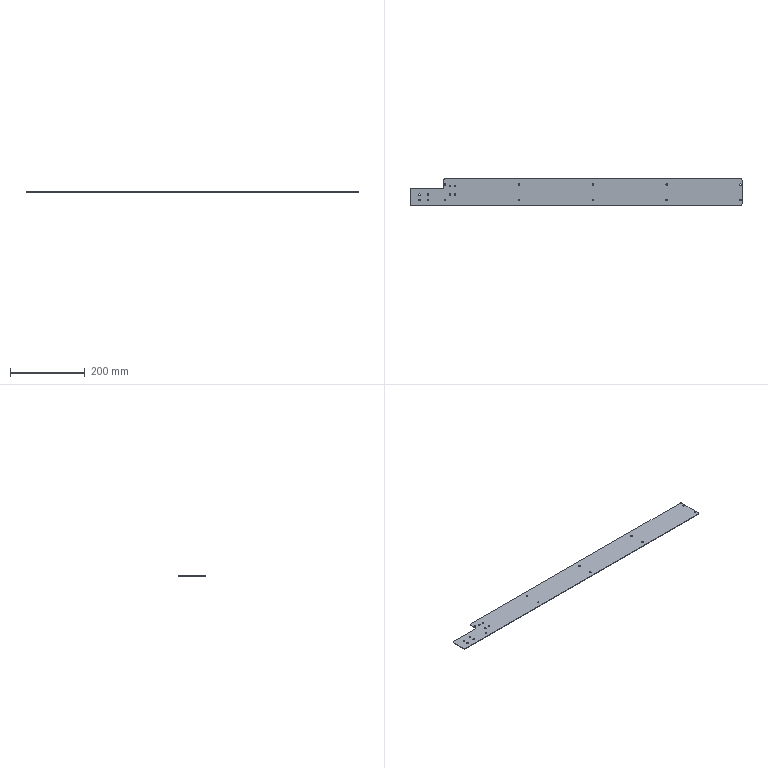Part | STEP file | SynoNew-0304-054 | 1 solid | 32 faces | box 890 x 70 x 1.5 mm | volume 89689 mm3 | cylinder 24 | plane 8 | commonest cylinder face diameters 4.2 x18 6 x6
STEP:
#1=CARTESIAN_POINT('',(-366.9,16.,1.5));
#2=VERTEX_POINT('',#1);
#3=CARTESIAN_POINT('',(-371.1,16.,1.5));
#4=VERTEX_POINT('',#3);
#5=CARTESIAN_POINT('',(-369.,16.,1.5));
#6=DIRECTION('',(0.,0.,-1.));
#7=DIRECTION('',(1.,0.,0.));
#8=AXIS2_PLACEMENT_3D('',#5,#6,#7);
#9=CIRCLE('',#8,2.1);
#10=EDGE_CURVE('',#2,#4,#9,.T.);
#11=ORIENTED_EDGE('',*,*,#10,.F.);
#12=CARTESIAN_POINT('',(-369.,16.,1.5));
#13=DIRECTION('',(0.,0.,-1.));
#14=DIRECTION('',(1.,0.,0.));
#15=AXIS2_PLACEMENT_3D('',#12,#13,#14);
#16=CIRCLE('',#15,2.1);
#17=EDGE_CURVE('',#4,#2,#16,.T.);
#18=ORIENTED_EDGE('',*,*,#17,.F.);
#19=CARTESIAN_POINT('',(-371.1,16.,0.));
#20=VERTEX_POINT('',#19);
#21=CARTESIAN_POINT('',(-371.1,16.,-2.5));
#22=DIRECTION('',(0.,0.,-1.));
#23=VECTOR('',#22,2.1);
#24=LINE('',#21,#23);
#25=EDGE_CURVE('',#4,#20,#24,.T.);
#26=ORIENTED_EDGE('',*,*,#25,.T.);
#27=CARTESIAN_POINT('',(-369.,16.,0.));
#28=DIRECTION('',(0.,0.,1.));
#29=DIRECTION('',(1.,0.,0.));
#30=AXIS2_PLACEMENT_3D('',#27,#28,#29);
#31=CIRCLE('',#30,2.1);
#32=EDGE_CURVE('',#20,#20,#31,.T.);
#33=ORIENTED_EDGE('',*,*,#32,.F.);
#34=ORIENTED_EDGE('',*,*,#25,.F.);
#35=EDGE_LOOP('',(#11,#18,#26,#33,#34));
#36=FACE_OUTER_BOUND('',#35,.T.);
#37=CARTESIAN_POINT('',(-369.,16.,-2.5));
#38=DIRECTION('',(0.,0.,1.));
#39=DIRECTION('',(1.,0.,0.));
#40=AXIS2_PLACEMENT_3D('',#37,#38,#39);
#41=CYLINDRICAL_SURFACE('',#40,2.1);
#42=ADVANCED_FACE('',(#36),#41,.F.);
#43=CARTESIAN_POINT('',(-380.9,-7.,1.5));
#44=VERTEX_POINT('',#43);
#45=CARTESIAN_POINT('',(-385.1,-7.,1.5));
#46=VERTEX_POINT('',#45);
#47=CARTESIAN_POINT('',(-383.,-7.,1.5));
#48=DIRECTION('',(0.,0.,-1.));
#49=DIRECTION('',(1.,0.,0.));
#50=AXIS2_PLACEMENT_3D('',#47,#48,#49);
#51=CIRCLE('',#50,2.1);
#52=EDGE_CURVE('',#44,#46,#51,.T.);
#53=ORIENTED_EDGE('',*,*,#52,.F.);
#54=CARTESIAN_POINT('',(-383.,-7.,1.5));
#55=DIRECTION('',(0.,0.,-1.));
#56=DIRECTION('',(1.,0.,0.));
#57=AXIS2_PLACEMENT_3D('',#54,#55,#56);
#58=CIRCLE('',#57,2.1);
#59=EDGE_CURVE('',#46,#44,#58,.T.);
#60=ORIENTED_EDGE('',*,*,#59,.F.);
#61=CARTESIAN_POINT('',(-385.1,-7.,0.));
#62=VERTEX_POINT('',#61);
#63=CARTESIAN_POINT('',(-385.1,-7.,-2.5));
#64=DIRECTION('',(0.,0.,-1.));
#65=VECTOR('',#64,2.1);
#66=LINE('',#63,#65);
#67=EDGE_CURVE('',#46,#62,#66,.T.);
#68=ORIENTED_EDGE('',*,*,#67,.T.);
#69=CARTESIAN_POINT('',(-383.,-7.,0.));
#70=DIRECTION('',(0.,0.,1.));
#71=DIRECTION('',(1.,0.,0.));
#72=AXIS2_PLACEMENT_3D('',#69,#70,#71);
#73=CIRCLE('',#72,2.1);
#74=EDGE_CURVE('',#62,#62,#73,.T.);
#75=ORIENTED_EDGE('',*,*,#74,.F.);
#76=ORIENTED_EDGE('',*,*,#67,.F.);
#77=EDGE_LOOP('',(#53,#60,#68,#75,#76));
#78=FACE_OUTER_BOUND('',#77,.T.);
#79=CARTESIAN_POINT('',(-383.,-7.,-2.5));
#80=DIRECTION('',(0.,0.,1.));
#81=DIRECTION('',(1.,0.,0.));
#82=AXIS2_PLACEMENT_3D('',#79,#80,#81);
#83=CYLINDRICAL_SURFACE('',#82,2.1);
#84=ADVANCED_FACE('',(#78),#83,.F.);
#85=CARTESIAN_POINT('',(-380.9,16.,1.5));
#86=VERTEX_POINT('',#85);
#87=CARTESIAN_POINT('',(-385.1,16.,1.5));
#88=VERTEX_POINT('',#87);
#89=CARTESIAN_POINT('',(-383.,16.,1.5));
#90=DIRECTION('',(0.,0.,-1.));
#91=DIRECTION('',(1.,0.,0.));
#92=AXIS2_PLACEMENT_3D('',#89,#90,#91);
#93=CIRCLE('',#92,2.1);
#94=EDGE_CURVE('',#86,#88,#93,.T.);
#95=ORIENTED_EDGE('',*,*,#94,.F.);
#96=CARTESIAN_POINT('',(-383.,16.,1.5));
#97=DIRECTION('',(0.,0.,-1.));
#98=DIRECTION('',(1.,0.,0.));
#99=AXIS2_PLACEMENT_3D('',#96,#97,#98);
#100=CIRCLE('',#99,2.1);
#101=EDGE_CURVE('',#88,#86,#100,.T.);
#102=ORIENTED_EDGE('',*,*,#101,.F.);
#103=CARTESIAN_POINT('',(-385.1,16.,0.));
#104=VERTEX_POINT('',#103);
#105=CARTESIAN_POINT('',(-385.1,16.,-2.5));
#106=DIRECTION('',(0.,0.,-1.));
#107=VECTOR('',#106,2.1);
#108=LINE('',#105,#107);
#109=EDGE_CURVE('',#88,#104,#108,.T.);
#110=ORIENTED_EDGE('',*,*,#109,.T.);
#111=CARTESIAN_POINT('',(-383.,16.,0.));
#112=DIRECTION('',(0.,0.,1.));
#113=DIRECTION('',(1.,0.,0.));
#114=AXIS2_PLACEMENT_3D('',#111,#112,#113);
#115=CIRCLE('',#114,2.1);
#116=EDGE_CURVE('',#104,#104,#115,.T.);
#117=ORIENTED_EDGE('',*,*,#116,.F.);
#118=ORIENTED_EDGE('',*,*,#109,.F.);
#119=EDGE_LOOP('',(#95,#102,#110,#117,#118));
#120=FACE_OUTER_BOUND('',#119,.T.);
#121=CARTESIAN_POINT('',(-383.,16.,-2.5));
#122=DIRECTION('',(0.,0.,1.));
#123=DIRECTION('',(1.,0.,0.));
#124=AXIS2_PLACEMENT_3D('',#121,#122,#123);
#125=CYLINDRICAL_SURFACE('',#124,2.1);
#126=ADVANCED_FACE('',(#120),#125,.F.);
#127=CARTESIAN_POINT('',(-366.9,-7.,1.5));
#128=VERTEX_POINT('',#127);
#129=CARTESIAN_POINT('',(-371.1,-7.,1.5));
#130=VERTEX_POINT('',#129);
#131=CARTESIAN_POINT('',(-369.,-7.,1.5));
#132=DIRECTION('',(0.,0.,-1.));
#133=DIRECTION('',(1.,0.,0.));
#134=AXIS2_PLACEMENT_3D('',#131,#132,#133);
#135=CIRCLE('',#134,2.1);
#136=EDGE_CURVE('',#128,#130,#135,.T.);
#137=ORIENTED_EDGE('',*,*,#136,.F.);
#138=CARTESIAN_POINT('',(-369.,-7.,1.5));
#139=DIRECTION('',(0.,0.,-1.));
#140=DIRECTION('',(1.,0.,0.));
#141=AXIS2_PLACEMENT_3D('',#138,#139,#140);
#142=CIRCLE('',#141,2.1);
#143=EDGE_CURVE('',#130,#128,#142,.T.);
#144=ORIENTED_EDGE('',*,*,#143,.F.);
#145=CARTESIAN_POINT('',(-371.1,-7.,0.));
#146=VERTEX_POINT('',#145);
#147=CARTESIAN_POINT('',(-371.1,-7.,-2.5));
#148=DIRECTION('',(0.,0.,-1.));
#149=VECTOR('',#148,2.1);
#150=LINE('',#147,#149);
#151=EDGE_CURVE('',#130,#146,#150,.T.);
#152=ORIENTED_EDGE('',*,*,#151,.T.);
#153=CARTESIAN_POINT('',(-369.,-7.,0.));
#154=DIRECTION('',(0.,0.,1.));
#155=DIRECTION('',(1.,0.,0.));
#156=AXIS2_PLACEMENT_3D('',#153,#154,#155);
#157=CIRCLE('',#156,2.1);
#158=EDGE_CURVE('',#146,#146,#157,.T.);
#159=ORIENTED_EDGE('',*,*,#158,.F.);
#160=ORIENTED_EDGE('',*,*,#151,.F.);
#161=EDGE_LOOP('',(#137,#144,#152,#159,#160));
#162=FACE_OUTER_BOUND('',#161,.T.);
#163=CARTESIAN_POINT('',(-369.,-7.,-2.5));
#164=DIRECTION('',(0.,0.,1.));
#165=DIRECTION('',(1.,0.,0.));
#166=AXIS2_PLACEMENT_3D('',#163,#164,#165);
#167=CYLINDRICAL_SURFACE('',#166,2.1);
#168=ADVANCED_FACE('',(#162),#167,.F.);
#169=CARTESIAN_POINT('',(397.,35.,1.5));
#170=VERTEX_POINT('',#169);
#171=CARTESIAN_POINT('',(400.,32.,1.5));
#172=VERTEX_POINT('',#171);
#173=CARTESIAN_POINT('',(397.,32.,1.5));
#174=DIRECTION('',(0.,0.,-1.));
#175=DIRECTION('',(0.7071,0.7071,0.));
#176=AXIS2_PLACEMENT_3D('',#173,#174,#175);
#177=CIRCLE('',#176,3.);
#178=EDGE_CURVE('',#170,#172,#177,.T.);
#179=ORIENTED_EDGE('',*,*,#178,.T.);
#180=CARTESIAN_POINT('',(400.,32.,0.));
#181=VERTEX_POINT('',#180);
#182=CARTESIAN_POINT('',(400.,32.,0.));
#183=DIRECTION('',(0.,0.,-1.));
#184=VECTOR('',#183,10.);
#185=LINE('',#182,#184);
#186=EDGE_CURVE('',#172,#181,#185,.T.);
#187=ORIENTED_EDGE('',*,*,#186,.T.);
#188=CARTESIAN_POINT('',(397.,35.,0.));
#189=VERTEX_POINT('',#188);
#190=CARTESIAN_POINT('',(397.,32.,0.));
#191=DIRECTION('',(0.,0.,1.));
#192=DIRECTION('',(0.7071,0.7071,0.));
#193=AXIS2_PLACEMENT_3D('',#190,#191,#192);
#194=CIRCLE('',#193,3.);
#195=EDGE_CURVE('',#181,#189,#194,.T.);
#196=ORIENTED_EDGE('',*,*,#195,.T.);
#197=CARTESIAN_POINT('',(397.,35.,0.));
#198=DIRECTION('',(0.,0.,1.));
#199=VECTOR('',#198,10.);
#200=LINE('',#197,#199);
#201=EDGE_CURVE('',#189,#170,#200,.T.);
#202=ORIENTED_EDGE('',*,*,#201,.T.);
#203=EDGE_LOOP('',(#179,#187,#196,#202));
#204=FACE_OUTER_BOUND('',#203,.T.);
#205=CARTESIAN_POINT('',(397.,32.,0.));
#206=DIRECTION('',(0.,0.,1.));
#207=DIRECTION('',(0.7071,0.7071,0.));
#208=AXIS2_PLACEMENT_3D('',#205,#206,#207);
#209=CYLINDRICAL_SURFACE('',#208,3.);
#210=ADVANCED_FACE('',(#204),#209,.T.);
#211=ORIENTED_EDGE('',*,*,#201,.F.);
#212=CARTESIAN_POINT('',(-397.,35.,0.));
#213=VERTEX_POINT('',#212);
#214=CARTESIAN_POINT('',(400.,35.,0.));
#215=DIRECTION('',(-1.,0.,0.));
#216=VECTOR('',#215,10.);
#217=LINE('',#214,#216);
#218=EDGE_CURVE('',#189,#213,#217,.T.);
#219=ORIENTED_EDGE('',*,*,#218,.T.);
#220=CARTESIAN_POINT('',(-397.,35.,1.5));
#221=VERTEX_POINT('',#220);
#222=CARTESIAN_POINT('',(-397.,35.,0.));
#223=DIRECTION('',(0.,0.,-1.));
#224=VECTOR('',#223,10.);
#225=LINE('',#222,#224);
#226=EDGE_CURVE('',#221,#213,#225,.T.);
#227=ORIENTED_EDGE('',*,*,#226,.F.);
#228=CARTESIAN_POINT('',(400.,35.,1.5));
#229=DIRECTION('',(-1.,0.,0.));
#230=VECTOR('',#229,10.);
#231=LINE('',#228,#230);
#232=EDGE_CURVE('',#170,#221,#231,.T.);
#233=ORIENTED_EDGE('',*,*,#232,.F.);
#234=EDGE_LOOP('',(#211,#219,#227,#233));
#235=FACE_OUTER_BOUND('',#234,.T.);
#236=CARTESIAN_POINT('',(400.,35.,0.));
#237=DIRECTION('',(0.,1.,0.));
#238=DIRECTION('',(-1.,0.,0.));
#239=AXIS2_PLACEMENT_3D('',#236,#237,#238);
#240=PLANE('',#239);
#241=ADVANCED_FACE('',(#235),#240,.T.);
#242=ORIENTED_EDGE('',*,*,#195,.F.);
#243=CARTESIAN_POINT('',(400.,-32.,0.));
#244=VERTEX_POINT('',#243);
#245=CARTESIAN_POINT('',(400.,-35.,0.));
#246=DIRECTION('',(0.,1.,0.));
#247=VECTOR('',#246,10.);
#248=LINE('',#245,#247);
#249=EDGE_CURVE('',#244,#181,#248,.T.);
#250=ORIENTED_EDGE('',*,*,#249,.F.);
#251=CARTESIAN_POINT('',(397.,-35.,0.));
#252=VERTEX_POINT('',#251);
#253=CARTESIAN_POINT('',(397.,-32.,0.));
#254=DIRECTION('',(0.,0.,1.));
#255=DIRECTION('',(0.7071,-0.7071,0.));
#256=AXIS2_PLACEMENT_3D('',#253,#254,#255);
#257=CIRCLE('',#256,3.);
#258=EDGE_CURVE('',#252,#244,#257,.T.);
#259=ORIENTED_EDGE('',*,*,#258,.F.);
#260=CARTESIAN_POINT('',(-487.,-35.,0.));
#261=VERTEX_POINT('',#260);
#262=CARTESIAN_POINT('',(-400.,-35.,0.));
#263=DIRECTION('',(-1.,0.,0.));
#264=VECTOR('',#263,10.);
#265=LINE('',#262,#264);
#266=EDGE_CURVE('',#252,#261,#265,.T.);
#267=ORIENTED_EDGE('',*,*,#266,.T.);
#268=CARTESIAN_POINT('',(-490.,-32.,0.));
#269=VERTEX_POINT('',#268);
#270=CARTESIAN_POINT('',(-487.,-32.,0.));
#271=DIRECTION('',(0.,0.,1.));
#272=DIRECTION('',(-0.7071,-0.7071,0.));
#273=AXIS2_PLACEMENT_3D('',#270,#271,#272);
#274=CIRCLE('',#273,3.);
#275=EDGE_CURVE('',#269,#261,#274,.T.);
#276=ORIENTED_EDGE('',*,*,#275,.F.);
#277=CARTESIAN_POINT('',(-490.,7.,0.));
#278=VERTEX_POINT('',#277);
#279=CARTESIAN_POINT('',(-490.,35.,0.));
#280=DIRECTION('',(0.,-1.,0.));
#281=VECTOR('',#280,10.);
#282=LINE('',#279,#281);
#283=EDGE_CURVE('',#278,#269,#282,.T.);
#284=ORIENTED_EDGE('',*,*,#283,.F.);
#285=CARTESIAN_POINT('',(-487.,10.,0.));
#286=VERTEX_POINT('',#285);
#287=CARTESIAN_POINT('',(-487.,7.,0.));
#288=DIRECTION('',(0.,0.,1.));
#289=DIRECTION('',(-0.7071,0.7071,0.));
#290=AXIS2_PLACEMENT_3D('',#287,#288,#289);
#291=CIRCLE('',#290,3.);
#292=EDGE_CURVE('',#286,#278,#291,.T.);
#293=ORIENTED_EDGE('',*,*,#292,.F.);
#294=CARTESIAN_POINT('',(-403.,10.,0.));
#295=VERTEX_POINT('',#294);
#296=CARTESIAN_POINT('',(-400.,10.,0.));
#297=DIRECTION('',(-1.,0.,0.));
#298=VECTOR('',#297,10.);
#299=LINE('',#296,#298);
#300=EDGE_CURVE('',#295,#286,#299,.T.);
#301=ORIENTED_EDGE('',*,*,#300,.F.);
#302=CARTESIAN_POINT('',(-400.,13.,0.));
#303=VERTEX_POINT('',#302);
#304=CARTESIAN_POINT('',(-403.,13.,0.));
#305=DIRECTION('',(0.,0.,-1.));
#306=DIRECTION('',(0.7071,-0.7071,0.));
#307=AXIS2_PLACEMENT_3D('',#304,#305,#306);
#308=CIRCLE('',#307,3.);
#309=EDGE_CURVE('',#303,#295,#308,.T.);
#310=ORIENTED_EDGE('',*,*,#309,.F.);
#311=CARTESIAN_POINT('',(-400.,32.,0.));
#312=VERTEX_POINT('',#311);
#313=CARTESIAN_POINT('',(-400.,35.,0.));
#314=DIRECTION('',(0.,-1.,0.));
#315=VECTOR('',#314,10.);
#316=LINE('',#313,#315);
#317=EDGE_CURVE('',#312,#303,#316,.T.);
#318=ORIENTED_EDGE('',*,*,#317,.F.);
#319=CARTESIAN_POINT('',(-397.,32.,0.));
#320=DIRECTION('',(0.,0.,1.));
#321=DIRECTION('',(-0.7071,0.7071,0.));
#322=AXIS2_PLACEMENT_3D('',#319,#320,#321);
#323=CIRCLE('',#322,3.);
#324=EDGE_CURVE('',#213,#312,#323,.T.);
#325=ORIENTED_EDGE('',*,*,#324,.F.);
#326=ORIENTED_EDGE('',*,*,#218,.F.);
#327=EDGE_LOOP('',(#242,#250,#259,#267,#276,#284,#293,#301,#310,#318,#325,#326));
#328=FACE_OUTER_BOUND('',#327,.T.);
#329=ORIENTED_EDGE('',*,*,#32,.T.);
#330=EDGE_LOOP('',(#329));
#331=FACE_BOUND('',#330,.T.);
#332=ORIENTED_EDGE('',*,*,#74,.T.);
#333=EDGE_LOOP('',(#332));
#334=FACE_BOUND('',#333,.T.);
#335=ORIENTED_EDGE('',*,*,#116,.T.);
#336=EDGE_LOOP('',(#335));
#337=FACE_BOUND('',#336,.T.);
#338=ORIENTED_EDGE('',*,*,#158,.T.);
#339=EDGE_LOOP('',(#338));
#340=FACE_BOUND('',#339,.T.);
#341=CARTESIAN_POINT('',(393.9,20.,0.));
#342=VERTEX_POINT('',#341);
#343=CARTESIAN_POINT('',(396.,20.,0.));
#344=DIRECTION('',(0.,0.,1.));
#345=DIRECTION('',(1.,0.,0.));
#346=AXIS2_PLACEMENT_3D('',#343,#344,#345);
#347=CIRCLE('',#346,2.1);
#348=EDGE_CURVE('',#342,#342,#347,.T.);
#349=ORIENTED_EDGE('',*,*,#348,.T.);
#350=EDGE_LOOP('',(#349));
#351=FACE_BOUND('',#350,.T.);
#352=CARTESIAN_POINT('',(393.9,-22.,0.));
#353=VERTEX_POINT('',#352);
#354=CARTESIAN_POINT('',(396.,-22.,0.));
#355=DIRECTION('',(0.,0.,1.));
#356=DIRECTION('',(1.,0.,0.));
#357=AXIS2_PLACEMENT_3D('',#354,#355,#356);
#358=CIRCLE('',#357,2.1);
#359=EDGE_CURVE('',#353,#353,#358,.T.);
#360=ORIENTED_EDGE('',*,*,#359,.T.);
#361=EDGE_LOOP('',(#360));
#362=FACE_BOUND('',#361,.T.);
#363=CARTESIAN_POINT('',(195.9,20.,0.));
#364=VERTEX_POINT('',#363);
#365=CARTESIAN_POINT('',(198.,20.,0.));
#366=DIRECTION('',(0.,0.,1.));
#367=DIRECTION('',(1.,0.,0.));
#368=AXIS2_PLACEMENT_3D('',#365,#366,#367);
#369=CIRCLE('',#368,2.1);
#370=EDGE_CURVE('',#364,#364,#369,.T.);
#371=ORIENTED_EDGE('',*,*,#370,.T.);
#372=EDGE_LOOP('',(#371));
#373=FACE_BOUND('',#372,.T.);
#374=CARTESIAN_POINT('',(195.9,-22.,0.));
#375=VERTEX_POINT('',#374);
#376=CARTESIAN_POINT('',(198.,-22.,0.));
#377=DIRECTION('',(0.,0.,1.));
#378=DIRECTION('',(1.,0.,0.));
#379=AXIS2_PLACEMENT_3D('',#376,#377,#378);
#380=CIRCLE('',#379,2.1);
#381=EDGE_CURVE('',#375,#375,#380,.T.);
#382=ORIENTED_EDGE('',*,*,#381,.T.);
#383=EDGE_LOOP('',(#382));
#384=FACE_BOUND('',#383,.T.);
#385=CARTESIAN_POINT('',(-2.1,20.,0.));
#386=VERTEX_POINT('',#385);
#387=CARTESIAN_POINT('',(0.,20.,0.));
#388=DIRECTION('',(0.,0.,1.));
#389=DIRECTION('',(1.,0.,0.));
#390=AXIS2_PLACEMENT_3D('',#387,#388,#389);
#391=CIRCLE('',#390,2.1);
#392=EDGE_CURVE('',#386,#386,#391,.T.);
#393=ORIENTED_EDGE('',*,*,#392,.T.);
#394=EDGE_LOOP('',(#393));
#395=FACE_BOUND('',#394,.T.);
#396=CARTESIAN_POINT('',(-2.1,-22.,0.));
#397=VERTEX_POINT('',#396);
#398=CARTESIAN_POINT('',(0.,-22.,0.));
#399=DIRECTION('',(0.,0.,1.));
#400=DIRECTION('',(1.,0.,0.));
#401=AXIS2_PLACEMENT_3D('',#398,#399,#400);
#402=CIRCLE('',#401,2.1);
#403=EDGE_CURVE('',#397,#397,#402,.T.);
#404=ORIENTED_EDGE('',*,*,#403,.T.);
#405=EDGE_LOOP('',(#404));
#406=FACE_BOUND('',#405,.T.);
#407=CARTESIAN_POINT('',(-200.1,20.,0.));
#408=VERTEX_POINT('',#407);
#409=CARTESIAN_POINT('',(-198.,20.,0.));
#410=DIRECTION('',(0.,0.,1.));
#411=DIRECTION('',(1.,0.,0.));
#412=AXIS2_PLACEMENT_3D('',#409,#410,#411);
#413=CIRCLE('',#412,2.1);
#414=EDGE_CURVE('',#408,#408,#413,.T.);
#415=ORIENTED_EDGE('',*,*,#414,.T.);
#416=EDGE_LOOP('',(#415));
#417=FACE_BOUND('',#416,.T.);
#418=CARTESIAN_POINT('',(-200.1,-22.,0.));
#419=VERTEX_POINT('',#418);
#420=CARTESIAN_POINT('',(-198.,-22.,0.));
#421=DIRECTION('',(0.,0.,1.));
#422=DIRECTION('',(1.,0.,0.));
#423=AXIS2_PLACEMENT_3D('',#420,#421,#422);
#424=CIRCLE('',#423,2.1);
#425=EDGE_CURVE('',#419,#419,#424,.T.);
#426=ORIENTED_EDGE('',*,*,#425,.T.);
#427=EDGE_LOOP('',(#426));
#428=FACE_BOUND('',#427,.T.);
#429=CARTESIAN_POINT('',(-398.1,20.,0.));
#430=VERTEX_POINT('',#429);
#431=CARTESIAN_POINT('',(-396.,20.,0.));
#432=DIRECTION('',(0.,0.,1.));
#433=DIRECTION('',(1.,0.,0.));
#434=AXIS2_PLACEMENT_3D('',#431,#432,#433);
#435=CIRCLE('',#434,2.1);
#436=EDGE_CURVE('',#430,#430,#435,.T.);
#437=ORIENTED_EDGE('',*,*,#436,.T.);
#438=EDGE_LOOP('',(#437));
#439=FACE_BOUND('',#438,.T.);
#440=CARTESIAN_POINT('',(-398.1,-22.,0.));
#441=VERTEX_POINT('',#440);
#442=CARTESIAN_POINT('',(-396.,-22.,0.));
#443=DIRECTION('',(0.,0.,1.));
#444=DIRECTION('',(1.,0.,0.));
#445=AXIS2_PLACEMENT_3D('',#442,#443,#444);
#446=CIRCLE('',#445,2.1);
#447=EDGE_CURVE('',#441,#441,#446,.T.);
#448=ORIENTED_EDGE('',*,*,#447,.T.);
#449=EDGE_LOOP('',(#448));
#450=FACE_BOUND('',#449,.T.);
#451=CARTESIAN_POINT('',(-466.6,-7.,0.));
#452=VERTEX_POINT('',#451);
#453=CARTESIAN_POINT('',(-464.5,-7.,0.));
#454=DIRECTION('',(0.,0.,1.));
#455=DIRECTION('',(1.,0.,0.));
#456=AXIS2_PLACEMENT_3D('',#453,#454,#455);
#457=CIRCLE('',#456,2.1);
#458=EDGE_CURVE('',#452,#452,#457,.T.);
#459=ORIENTED_EDGE('',*,*,#458,.T.);
#460=EDGE_LOOP('',(#459));
#461=FACE_BOUND('',#460,.T.);
#462=CARTESIAN_POINT('',(-443.6,-21.,0.));
#463=VERTEX_POINT('',#462);
#464=CARTESIAN_POINT('',(-441.5,-21.,0.));
#465=DIRECTION('',(0.,0.,1.));
#466=DIRECTION('',(1.,0.,0.));
#467=AXIS2_PLACEMENT_3D('',#464,#465,#466);
#468=CIRCLE('',#467,2.1);
#469=EDGE_CURVE('',#463,#463,#468,.T.);
#470=ORIENTED_EDGE('',*,*,#469,.T.);
#471=EDGE_LOOP('',(#470));
#472=FACE_BOUND('',#471,.T.);
#473=CARTESIAN_POINT('',(-443.6,-7.,0.));
#474=VERTEX_POINT('',#473);
#475=CARTESIAN_POINT('',(-441.5,-7.,0.));
#476=DIRECTION('',(0.,0.,1.));
#477=DIRECTION('',(1.,0.,0.));
#478=AXIS2_PLACEMENT_3D('',#475,#476,#477);
#479=CIRCLE('',#478,2.1);
#480=EDGE_CURVE('',#474,#474,#479,.T.);
#481=ORIENTED_EDGE('',*,*,#480,.T.);
#482=EDGE_LOOP('',(#481));
#483=FACE_BOUND('',#482,.T.);
#484=CARTESIAN_POINT('',(-466.6,-21.,0.));
#485=VERTEX_POINT('',#484);
#486=CARTESIAN_POINT('',(-464.5,-21.,0.));
#487=DIRECTION('',(0.,0.,1.));
#488=DIRECTION('',(1.,0.,0.));
#489=AXIS2_PLACEMENT_3D('',#486,#487,#488);
#490=CIRCLE('',#489,2.1);
#491=EDGE_CURVE('',#485,#485,#490,.T.);
#492=ORIENTED_EDGE('',*,*,#491,.T.);
#493=EDGE_LOOP('',(#492));
#494=FACE_BOUND('',#493,.T.);
#495=CARTESIAN_POINT('',(0.,0.,0.));
#496=DIRECTION('',(0.,0.,1.));
#497=DIRECTION('',(1.,0.,0.));
#498=AXIS2_PLACEMENT_3D('',#495,#496,#497);
#499=PLANE('',#498);
#500=ADVANCED_FACE('',(#328,#331,#334,#337,#340,#351,#362,#373,#384,#395,#406,#417,#428,#439,#450,#461,#472,#483,#494),#499,.F.);
#501=CARTESIAN_POINT('',(400.,-32.,1.5));
#502=VERTEX_POINT('',#501);
#503=CARTESIAN_POINT('',(397.,-35.,1.5));
#504=VERTEX_POINT('',#503);
#505=CARTESIAN_POINT('',(397.,-32.,1.5));
#506=DIRECTION('',(0.,0.,-1.));
#507=DIRECTION('',(0.7071,-0.7071,0.));
#508=AXIS2_PLACEMENT_3D('',#505,#506,#507);
#509=CIRCLE('',#508,3.);
#510=EDGE_CURVE('',#502,#504,#509,.T.);
#511=ORIENTED_EDGE('',*,*,#510,.T.);
#512=CARTESIAN_POINT('',(397.,-35.,0.));
#513=DIRECTION('',(0.,0.,-1.));
#514=VECTOR('',#513,10.);
#515=LINE('',#512,#514);
#516=EDGE_CURVE('',#504,#252,#515,.T.);
#517=ORIENTED_EDGE('',*,*,#516,.T.);
#518=ORIENTED_EDGE('',*,*,#258,.T.);
#519=CARTESIAN_POINT('',(400.,-32.,0.));
#520=DIRECTION('',(0.,0.,1.));
#521=VECTOR('',#520,10.);
#522=LINE('',#519,#521);
#523=EDGE_CURVE('',#244,#502,#522,.T.);
#524=ORIENTED_EDGE('',*,*,#523,.T.);
#525=EDGE_LOOP('',(#511,#517,#518,#524));
#526=FACE_OUTER_BOUND('',#525,.T.);
#527=CARTESIAN_POINT('',(397.,-32.,0.));
#528=DIRECTION('',(0.,0.,1.));
#529=DIRECTION('',(0.7071,-0.7071,0.));
#530=AXIS2_PLACEMENT_3D('',#527,#528,#529);
#531=CYLINDRICAL_SURFACE('',#530,3.);
#532=ADVANCED_FACE('',(#526),#531,.T.);
#533=ORIENTED_EDGE('',*,*,#516,.F.);
#534=CARTESIAN_POINT('',(-487.,-35.,1.5));
#535=VERTEX_POINT('',#534);
#536=CARTESIAN_POINT('',(-400.,-35.,1.5));
#537=DIRECTION('',(-1.,0.,0.));
#538=VECTOR('',#537,10.);
#539=LINE('',#536,#538);
#540=EDGE_CURVE('',#504,#535,#539,.T.);
#541=ORIENTED_EDGE('',*,*,#540,.T.);
#542=CARTESIAN_POINT('',(-487.,-35.,0.375));
#543=DIRECTION('',(0.,0.,1.));
#544=VECTOR('',#543,10.);
#545=LINE('',#542,#544);
#546=EDGE_CURVE('',#261,#535,#545,.T.);
#547=ORIENTED_EDGE('',*,*,#546,.F.);
#548=ORIENTED_EDGE('',*,*,#266,.F.);
#549=EDGE_LOOP('',(#533,#541,#547,#548));
#550=FACE_OUTER_BOUND('',#549,.T.);
#551=CARTESIAN_POINT('',(-400.,-35.,0.));
#552=DIRECTION('',(0.,-1.,0.));
#553=DIRECTION('',(1.,0.,0.));
#554=AXIS2_PLACEMENT_3D('',#551,#552,#553);
#555=PLANE('',#554);
#556=ADVANCED_FACE('',(#550),#555,.T.);
#557=CARTESIAN_POINT('',(-490.,-32.,1.5));
#558=VERTEX_POINT('',#557);
#559=CARTESIAN_POINT('',(-487.,-32.,1.5));
#560=DIRECTION('',(0.,0.,-1.));
#561=DIRECTION('',(-0.7071,-0.7071,0.));
#562=AXIS2_PLACEMENT_3D('',#559,#560,#561);
#563=CIRCLE('',#562,3.);
#564=EDGE_CURVE('',#535,#558,#563,.T.);
#565=ORIENTED_EDGE('',*,*,#564,.T.);
#566=CARTESIAN_POINT('',(-490.,-32.,0.375));
#567=DIRECTION('',(0.,0.,-1.));
#568=VECTOR('',#567,10.);
#569=LINE('',#566,#568);
#570=EDGE_CURVE('',#558,#269,#569,.T.);
#571=ORIENTED_EDGE('',*,*,#570,.T.);
#572=ORIENTED_EDGE('',*,*,#275,.T.);
#573=ORIENTED_EDGE('',*,*,#546,.T.);
#574=EDGE_LOOP('',(#565,#571,#572,#573));
#575=FACE_OUTER_BOUND('',#574,.T.);
#576=CARTESIAN_POINT('',(-487.,-32.,0.375));
#577=DIRECTION('',(0.,0.,1.));
#578=DIRECTION('',(-0.7071,-0.7071,0.));
#579=AXIS2_PLACEMENT_3D('',#576,#577,#578);
#580=CYLINDRICAL_SURFACE('',#579,3.);
#581=ADVANCED_FACE('',(#575),#580,.T.);
#582=ORIENTED_EDGE('',*,*,#292,.T.);
#583=CARTESIAN_POINT('',(-490.,7.,1.5));
#584=VERTEX_POINT('',#583);
#585=CARTESIAN_POINT('',(-490.,7.,1.125));
#586=DIRECTION('',(0.,0.,1.));
#587=VECTOR('',#586,10.);
#588=LINE('',#585,#587);
#589=EDGE_CURVE('',#278,#584,#588,.T.);
#590=ORIENTED_EDGE('',*,*,#589,.T.);
#591=CARTESIAN_POINT('',(-487.,10.,1.5));
#592=VERTEX_POINT('',#591);
#593=CARTESIAN_POINT('',(-487.,7.,1.5));
#594=DIRECTION('',(0.,0.,-1.));
#595=DIRECTION('',(-0.7071,0.7071,0.));
#596=AXIS2_PLACEMENT_3D('',#593,#594,#595);
#597=CIRCLE('',#596,3.);
#598=EDGE_CURVE('',#584,#592,#597,.T.);
#599=ORIENTED_EDGE('',*,*,#598,.T.);
#600=CARTESIAN_POINT('',(-487.,10.,1.125));
#601=DIRECTION('',(0.,0.,-1.));
#602=VECTOR('',#601,10.);
#603=LINE('',#600,#602);
#604=EDGE_CURVE('',#592,#286,#603,.T.);
#605=ORIENTED_EDGE('',*,*,#604,.T.);
#606=EDGE_LOOP('',(#582,#590,#599,#605));
#607=FACE_OUTER_BOUND('',#606,.T.);
#608=CARTESIAN_POINT('',(-487.,7.,1.125));
#609=DIRECTION('',(0.,0.,-1.));
#610=DIRECTION('',(-0.7071,0.7071,0.));
#611=AXIS2_PLACEMENT_3D('',#608,#609,#610);
#612=CYLINDRICAL_SURFACE('',#611,3.);
#613=ADVANCED_FACE('',(#607),#612,.T.);
#614=ORIENTED_EDGE('',*,*,#604,.F.);
#615=CARTESIAN_POINT('',(-403.,10.,1.5));
#616=VERTEX_POINT('',#615);
#617=CARTESIAN_POINT('',(-400.,10.,1.5));
#618=DIRECTION('',(-1.,0.,0.));
#619=VECTOR('',#618,10.);
#620=LINE('',#617,#619);
#621=EDGE_CURVE('',#616,#592,#620,.T.);
#622=ORIENTED_EDGE('',*,*,#621,.F.);
#623=CARTESIAN_POINT('',(-403.,10.,0.75));
#624=DIRECTION('',(0.,0.,1.));
#625=VECTOR('',#624,10.);
#626=LINE('',#623,#625);
#627=EDGE_CURVE('',#295,#616,#626,.T.);
#628=ORIENTED_EDGE('',*,*,#627,.F.);
#629=ORIENTED_EDGE('',*,*,#300,.T.);
#630=EDGE_LOOP('',(#614,#622,#628,#629));
#631=FACE_OUTER_BOUND('',#630,.T.);
#632=CARTESIAN_POINT('',(-400.,10.,1.5));
#633=DIRECTION('',(0.,1.,0.));
#634=DIRECTION('',(0.,0.,-1.));
#635=AXIS2_PLACEMENT_3D('',#632,#633,#634);
#636=PLANE('',#635);
#637=ADVANCED_FACE('',(#631),#636,.T.);
#638=ORIENTED_EDGE('',*,*,#309,.T.);
#639=ORIENTED_EDGE('',*,*,#627,.T.);
#640=CARTESIAN_POINT('',(-400.,13.,1.5));
#641=VERTEX_POINT('',#640);
#642=CARTESIAN_POINT('',(-403.,13.,1.5));
#643=DIRECTION('',(0.,0.,1.));
#644=DIRECTION('',(0.7071,-0.7071,0.));
#645=AXIS2_PLACEMENT_3D('',#642,#643,#644);
#646=CIRCLE('',#645,3.);
#647=EDGE_CURVE('',#616,#641,#646,.T.);
#648=ORIENTED_EDGE('',*,*,#647,.T.);
#649=CARTESIAN_POINT('',(-400.,13.,0.75));
#650=DIRECTION('',(0.,0.,-1.));
#651=VECTOR('',#650,10.);
#652=LINE('',#649,#651);
#653=EDGE_CURVE('',#641,#303,#652,.T.);
#654=ORIENTED_EDGE('',*,*,#653,.T.);
#655=EDGE_LOOP('',(#638,#639,#648,#654));
#656=FACE_OUTER_BOUND('',#655,.T.);
#657=CARTESIAN_POINT('',(-403.,13.,0.75));
#658=DIRECTION('',(0.,0.,1.));
#659=DIRECTION('',(0.7071,-0.7071,0.));
#660=AXIS2_PLACEMENT_3D('',#657,#658,#659);
#661=CYLINDRICAL_SURFACE('',#660,3.);
#662=ADVANCED_FACE('',(#656),#661,.F.);
#663=CARTESIAN_POINT('',(-400.,32.,1.5));
#664=VERTEX_POINT('',#663);
#665=CARTESIAN_POINT('',(-397.,32.,1.5));
#666=DIRECTION('',(0.,0.,-1.));
#667=DIRECTION('',(-0.7071,0.7071,0.));
#668=AXIS2_PLACEMENT_3D('',#665,#666,#667);
#669=CIRCLE('',#668,3.);
#670=EDGE_CURVE('',#664,#221,#669,.T.);
#671=ORIENTED_EDGE('',*,*,#670,.T.);
#672=ORIENTED_EDGE('',*,*,#226,.T.);
#673=ORIENTED_EDGE('',*,*,#324,.T.);
#674=CARTESIAN_POINT('',(-400.,32.,0.));
#675=DIRECTION('',(0.,0.,1.));
#676=VECTOR('',#675,10.);
#677=LINE('',#674,#676);
#678=EDGE_CURVE('',#312,#664,#677,.T.);
#679=ORIENTED_EDGE('',*,*,#678,.T.);
#680=EDGE_LOOP('',(#671,#672,#673,#679));
#681=FACE_OUTER_BOUND('',#680,.T.);
#682=CARTESIAN_POINT('',(-397.,32.,0.));
#683=DIRECTION('',(0.,0.,1.));
#684=DIRECTION('',(-0.7071,0.7071,0.));
#685=AXIS2_PLACEMENT_3D('',#682,#683,#684);
#686=CYLINDRICAL_SURFACE('',#685,3.);
#687=ADVANCED_FACE('',(#681),#686,.T.);
#688=CARTESIAN_POINT('',(-462.4,-21.,1.5));
#689=VERTEX_POINT('',#688);
#690=CARTESIAN_POINT('',(-466.6,-21.,1.5));
#691=VERTEX_POINT('',#690);
#692=CARTESIAN_POINT('',(-464.5,-21.,1.5));
#693=DIRECTION('',(0.,0.,-1.));
#694=DIRECTION('',(1.,0.,0.));
#695=AXIS2_PLACEMENT_3D('',#692,#693,#694);
#696=CIRCLE('',#695,2.1);
#697=EDGE_CURVE('',#689,#691,#696,.T.);
#698=ORIENTED_EDGE('',*,*,#697,.F.);
#699=CARTESIAN_POINT('',(-464.5,-21.,1.5));
#700=DIRECTION('',(0.,0.,-1.));
#701=DIRECTION('',(1.,0.,0.));
#702=AXIS2_PLACEMENT_3D('',#699,#700,#701);
#703=CIRCLE('',#702,2.1);
#704=EDGE_CURVE('',#691,#689,#703,.T.);
#705=ORIENTED_EDGE('',*,*,#704,.F.);
#706=CARTESIAN_POINT('',(-466.6,-21.,-2.5));
#707=DIRECTION('',(0.,0.,-1.));
#708=VECTOR('',#707,2.1);
#709=LINE('',#706,#708);
#710=EDGE_CURVE('',#691,#485,#709,.T.);
#711=ORIENTED_EDGE('',*,*,#710,.T.);
#712=ORIENTED_EDGE('',*,*,#491,.F.);
#713=ORIENTED_EDGE('',*,*,#710,.F.);
#714=EDGE_LOOP('',(#698,#705,#711,#712,#713));
#715=FACE_OUTER_BOUND('',#714,.T.);
#716=CARTESIAN_POINT('',(-464.5,-21.,-2.5));
#717=DIRECTION('',(0.,0.,1.));
#718=DIRECTION('',(1.,0.,0.));
#719=AXIS2_PLACEMENT_3D('',#716,#717,#718);
#720=CYLINDRICAL_SURFACE('',#719,2.1);
#721=ADVANCED_FACE('',(#715),#720,.F.);
#722=CARTESIAN_POINT('',(-439.4,-7.,1.5));
#723=VERTEX_POINT('',#722);
#724=CARTESIAN_POINT('',(-443.6,-7.,1.5));
#725=VERTEX_POINT('',#724);
#726=CARTESIAN_POINT('',(-441.5,-7.,1.5));
#727=DIRECTION('',(0.,0.,-1.));
#728=DIRECTION('',(1.,0.,0.));
#729=AXIS2_PLACEMENT_3D('',#726,#727,#728);
#730=CIRCLE('',#729,2.1);
#731=EDGE_CURVE('',#723,#725,#730,.T.);
#732=ORIENTED_EDGE('',*,*,#731,.F.);
#733=CARTESIAN_POINT('',(-441.5,-7.,1.5));
#734=DIRECTION('',(0.,0.,-1.));
#735=DIRECTION('',(1.,0.,0.));
#736=AXIS2_PLACEMENT_3D('',#733,#734,#735);
#737=CIRCLE('',#736,2.1);
#738=EDGE_CURVE('',#725,#723,#737,.T.);
#739=ORIENTED_EDGE('',*,*,#738,.F.);
#740=CARTESIAN_POINT('',(-443.6,-7.,-2.5));
#741=DIRECTION('',(0.,0.,-1.));
#742=VECTOR('',#741,2.1);
#743=LINE('',#740,#742);
#744=EDGE_CURVE('',#725,#474,#743,.T.);
#745=ORIENTED_EDGE('',*,*,#744,.T.);
#746=ORIENTED_EDGE('',*,*,#480,.F.);
#747=ORIENTED_EDGE('',*,*,#744,.F.);
#748=EDGE_LOOP('',(#732,#739,#745,#746,#747));
#749=FACE_OUTER_BOUND('',#748,.T.);
#750=CARTESIAN_POINT('',(-441.5,-7.,-2.5));
#751=DIRECTION('',(0.,0.,1.));
#752=DIRECTION('',(1.,0.,0.));
#753=AXIS2_PLACEMENT_3D('',#750,#751,#752);
#754=CYLINDRICAL_SURFACE('',#753,2.1);
#755=ADVANCED_FACE('',(#749),#754,.F.);
#756=CARTESIAN_POINT('',(-439.4,-21.,1.5));
#757=VERTEX_POINT('',#756);
#758=CARTESIAN_POINT('',(-443.6,-21.,1.5));
#759=VERTEX_POINT('',#758);
#760=CARTESIAN_POINT('',(-441.5,-21.,1.5));
#761=DIRECTION('',(0.,0.,-1.));
#762=DIRECTION('',(1.,0.,0.));
#763=AXIS2_PLACEMENT_3D('',#760,#761,#762);
#764=CIRCLE('',#763,2.1);
#765=EDGE_CURVE('',#757,#759,#764,.T.);
#766=ORIENTED_EDGE('',*,*,#765,.F.);
#767=CARTESIAN_POINT('',(-441.5,-21.,1.5));
#768=DIRECTION('',(0.,0.,-1.));
#769=DIRECTION('',(1.,0.,0.));
#770=AXIS2_PLACEMENT_3D('',#767,#768,#769);
#771=CIRCLE('',#770,2.1);
#772=EDGE_CURVE('',#759,#757,#771,.T.);
#773=ORIENTED_EDGE('',*,*,#772,.F.);
#774=CARTESIAN_POINT('',(-443.6,-21.,-2.5));
#775=DIRECTION('',(0.,0.,-1.));
#776=VECTOR('',#775,2.1);
#777=LINE('',#774,#776);
#778=EDGE_CURVE('',#759,#463,#777,.T.);
#779=ORIENTED_EDGE('',*,*,#778,.T.);
#780=ORIENTED_EDGE('',*,*,#469,.F.);
#781=ORIENTED_EDGE('',*,*,#778,.F.);
#782=EDGE_LOOP('',(#766,#773,#779,#780,#781));
#783=FACE_OUTER_BOUND('',#782,.T.);
#784=CARTESIAN_POINT('',(-441.5,-21.,-2.5));
#785=DIRECTION('',(0.,0.,1.));
#786=DIRECTION('',(1.,0.,0.));
#787=AXIS2_PLACEMENT_3D('',#784,#785,#786);
#788=CYLINDRICAL_SURFACE('',#787,2.1);
#789=ADVANCED_FACE('',(#783),#788,.F.);
#790=CARTESIAN_POINT('',(-462.4,-7.,1.5));
#791=VERTEX_POINT('',#790);
#792=CARTESIAN_POINT('',(-466.6,-7.,1.5));
#793=VERTEX_POINT('',#792);
#794=CARTESIAN_POINT('',(-464.5,-7.,1.5));
#795=DIRECTION('',(0.,0.,-1.));
#796=DIRECTION('',(1.,0.,0.));
#797=AXIS2_PLACEMENT_3D('',#794,#795,#796);
#798=CIRCLE('',#797,2.1);
#799=EDGE_CURVE('',#791,#793,#798,.T.);
#800=ORIENTED_EDGE('',*,*,#799,.F.);
#801=CARTESIAN_POINT('',(-464.5,-7.,1.5));
#802=DIRECTION('',(0.,0.,-1.));
#803=DIRECTION('',(1.,0.,0.));
#804=AXIS2_PLACEMENT_3D('',#801,#802,#803);
#805=CIRCLE('',#804,2.1);
#806=EDGE_CURVE('',#793,#791,#805,.T.);
#807=ORIENTED_EDGE('',*,*,#806,.F.);
#808=CARTESIAN_POINT('',(-466.6,-7.,-2.5));
#809=DIRECTION('',(0.,0.,-1.));
#810=VECTOR('',#809,2.1);
#811=LINE('',#808,#810);
#812=EDGE_CURVE('',#793,#452,#811,.T.);
#813=ORIENTED_EDGE('',*,*,#812,.T.);
#814=ORIENTED_EDGE('',*,*,#458,.F.);
#815=ORIENTED_EDGE('',*,*,#812,.F.);
#816=EDGE_LOOP('',(#800,#807,#813,#814,#815));
#817=FACE_OUTER_BOUND('',#816,.T.);
#818=CARTESIAN_POINT('',(-464.5,-7.,-2.5));
#819=DIRECTION('',(0.,0.,1.));
#820=DIRECTION('',(1.,0.,0.));
#821=AXIS2_PLACEMENT_3D('',#818,#819,#820);
#822=CYLINDRICAL_SURFACE('',#821,2.1);
#823=ADVANCED_FACE('',(#817),#822,.F.);
#824=CARTESIAN_POINT('',(-393.9,-22.,1.5));
#825=VERTEX_POINT('',#824);
#826=CARTESIAN_POINT('',(-398.1,-22.,1.5));
#827=VERTEX_POINT('',#826);
#828=CARTESIAN_POINT('',(-396.,-22.,1.5));
#829=DIRECTION('',(0.,0.,-1.));
#830=DIRECTION('',(1.,0.,0.));
#831=AXIS2_PLACEMENT_3D('',#828,#829,#830);
#832=CIRCLE('',#831,2.1);
#833=EDGE_CURVE('',#825,#827,#832,.T.);
#834=ORIENTED_EDGE('',*,*,#833,.F.);
#835=CARTESIAN_POINT('',(-396.,-22.,1.5));
#836=DIRECTION('',(0.,0.,-1.));
#837=DIRECTION('',(1.,0.,0.));
#838=AXIS2_PLACEMENT_3D('',#835,#836,#837);
#839=CIRCLE('',#838,2.1);
#840=EDGE_CURVE('',#827,#825,#839,.T.);
#841=ORIENTED_EDGE('',*,*,#840,.F.);
#842=CARTESIAN_POINT('',(-398.1,-22.,-2.5));
#843=DIRECTION('',(0.,0.,-1.));
#844=VECTOR('',#843,2.1);
#845=LINE('',#842,#844);
#846=EDGE_CURVE('',#827,#441,#845,.T.);
#847=ORIENTED_EDGE('',*,*,#846,.T.);
#848=ORIENTED_EDGE('',*,*,#447,.F.);
#849=ORIENTED_EDGE('',*,*,#846,.F.);
#850=EDGE_LOOP('',(#834,#841,#847,#848,#849));
#851=FACE_OUTER_BOUND('',#850,.T.);
#852=CARTESIAN_POINT('',(-396.,-22.,-2.5));
#853=DIRECTION('',(0.,0.,1.));
#854=DIRECTION('',(1.,0.,0.));
#855=AXIS2_PLACEMENT_3D('',#852,#853,#854);
#856=CYLINDRICAL_SURFACE('',#855,2.1);
#857=ADVANCED_FACE('',(#851),#856,.F.);
#858=CARTESIAN_POINT('',(-393.9,20.,1.5));
#859=VERTEX_POINT('',#858);
#860=CARTESIAN_POINT('',(-398.1,20.,1.5));
#861=VERTEX_POINT('',#860);
#862=CARTESIAN_POINT('',(-396.,20.,1.5));
#863=DIRECTION('',(0.,0.,-1.));
#864=DIRECTION('',(1.,0.,0.));
#865=AXIS2_PLACEMENT_3D('',#862,#863,#864);
#866=CIRCLE('',#865,2.1);
#867=EDGE_CURVE('',#859,#861,#866,.T.);
#868=ORIENTED_EDGE('',*,*,#867,.F.);
#869=CARTESIAN_POINT('',(-396.,20.,1.5));
#870=DIRECTION('',(0.,0.,-1.));
#871=DIRECTION('',(1.,0.,0.));
#872=AXIS2_PLACEMENT_3D('',#869,#870,#871);
#873=CIRCLE('',#872,2.1);
#874=EDGE_CURVE('',#861,#859,#873,.T.);
#875=ORIENTED_EDGE('',*,*,#874,.F.);
#876=CARTESIAN_POINT('',(-398.1,20.,-2.5));
#877=DIRECTION('',(0.,0.,-1.));
#878=VECTOR('',#877,2.1);
#879=LINE('',#876,#878);
#880=EDGE_CURVE('',#861,#430,#879,.T.);
#881=ORIENTED_EDGE('',*,*,#880,.T.);
#882=ORIENTED_EDGE('',*,*,#436,.F.);
#883=ORIENTED_EDGE('',*,*,#880,.F.);
#884=EDGE_LOOP('',(#868,#875,#881,#882,#883));
#885=FACE_OUTER_BOUND('',#884,.T.);
#886=CARTESIAN_POINT('',(-396.,20.,-2.5));
#887=DIRECTION('',(0.,0.,1.));
#888=DIRECTION('',(1.,0.,0.));
#889=AXIS2_PLACEMENT_3D('',#886,#887,#888);
#890=CYLINDRICAL_SURFACE('',#889,2.1);
#891=ADVANCED_FACE('',(#885),#890,.F.);
#892=CARTESIAN_POINT('',(-195.9,-22.,1.5));
#893=VERTEX_POINT('',#892);
#894=CARTESIAN_POINT('',(-200.1,-22.,1.5));
#895=VERTEX_POINT('',#894);
#896=CARTESIAN_POINT('',(-198.,-22.,1.5));
#897=DIRECTION('',(0.,0.,-1.));
#898=DIRECTION('',(1.,0.,0.));
#899=AXIS2_PLACEMENT_3D('',#896,#897,#898);
#900=CIRCLE('',#899,2.1);
#901=EDGE_CURVE('',#893,#895,#900,.T.);
#902=ORIENTED_EDGE('',*,*,#901,.F.);
#903=CARTESIAN_POINT('',(-198.,-22.,1.5));
#904=DIRECTION('',(0.,0.,-1.));
#905=DIRECTION('',(1.,0.,0.));
#906=AXIS2_PLACEMENT_3D('',#903,#904,#905);
#907=CIRCLE('',#906,2.1);
#908=EDGE_CURVE('',#895,#893,#907,.T.);
#909=ORIENTED_EDGE('',*,*,#908,.F.);
#910=CARTESIAN_POINT('',(-200.1,-22.,-2.5));
#911=DIRECTION('',(0.,0.,-1.));
#912=VECTOR('',#911,2.1);
#913=LINE('',#910,#912);
#914=EDGE_CURVE('',#895,#419,#913,.T.);
#915=ORIENTED_EDGE('',*,*,#914,.T.);
#916=ORIENTED_EDGE('',*,*,#425,.F.);
#917=ORIENTED_EDGE('',*,*,#914,.F.);
#918=EDGE_LOOP('',(#902,#909,#915,#916,#917));
#919=FACE_OUTER_BOUND('',#918,.T.);
#920=CARTESIAN_POINT('',(-198.,-22.,-2.5));
#921=DIRECTION('',(0.,0.,1.));
#922=DIRECTION('',(1.,0.,0.));
#923=AXIS2_PLACEMENT_3D('',#920,#921,#922);
#924=CYLINDRICAL_SURFACE('',#923,2.1);
#925=ADVANCED_FACE('',(#919),#924,.F.);
#926=CARTESIAN_POINT('',(-195.9,20.,1.5));
#927=VERTEX_POINT('',#926);
#928=CARTESIAN_POINT('',(-200.1,20.,1.5));
#929=VERTEX_POINT('',#928);
#930=CARTESIAN_POINT('',(-198.,20.,1.5));
#931=DIRECTION('',(0.,0.,-1.));
#932=DIRECTION('',(1.,0.,0.));
#933=AXIS2_PLACEMENT_3D('',#930,#931,#932);
#934=CIRCLE('',#933,2.1);
#935=EDGE_CURVE('',#927,#929,#934,.T.);
#936=ORIENTED_EDGE('',*,*,#935,.F.);
#937=CARTESIAN_POINT('',(-198.,20.,1.5));
#938=DIRECTION('',(0.,0.,-1.));
#939=DIRECTION('',(1.,0.,0.));
#940=AXIS2_PLACEMENT_3D('',#937,#938,#939);
#941=CIRCLE('',#940,2.1);
#942=EDGE_CURVE('',#929,#927,#941,.T.);
#943=ORIENTED_EDGE('',*,*,#942,.F.);
#944=CARTESIAN_POINT('',(-200.1,20.,-2.5));
#945=DIRECTION('',(0.,0.,-1.));
#946=VECTOR('',#945,2.1);
#947=LINE('',#944,#946);
#948=EDGE_CURVE('',#929,#408,#947,.T.);
#949=ORIENTED_EDGE('',*,*,#948,.T.);
#950=ORIENTED_EDGE('',*,*,#414,.F.);
#951=ORIENTED_EDGE('',*,*,#948,.F.);
#952=EDGE_LOOP('',(#936,#943,#949,#950,#951));
#953=FACE_OUTER_BOUND('',#952,.T.);
#954=CARTESIAN_POINT('',(-198.,20.,-2.5));
#955=DIRECTION('',(0.,0.,1.));
#956=DIRECTION('',(1.,0.,0.));
#957=AXIS2_PLACEMENT_3D('',#954,#955,#956);
#958=CYLINDRICAL_SURFACE('',#957,2.1);
#959=ADVANCED_FACE('',(#953),#958,.F.);
#960=CARTESIAN_POINT('',(2.1,-22.,1.5));
#961=VERTEX_POINT('',#960);
#962=CARTESIAN_POINT('',(-2.1,-22.,1.5));
#963=VERTEX_POINT('',#962);
#964=CARTESIAN_POINT('',(0.,-22.,1.5));
#965=DIRECTION('',(0.,0.,-1.));
#966=DIRECTION('',(1.,0.,0.));
#967=AXIS2_PLACEMENT_3D('',#964,#965,#966);
#968=CIRCLE('',#967,2.1);
#969=EDGE_CURVE('',#961,#963,#968,.T.);
#970=ORIENTED_EDGE('',*,*,#969,.F.);
#971=CARTESIAN_POINT('',(0.,-22.,1.5));
#972=DIRECTION('',(0.,0.,-1.));
#973=DIRECTION('',(1.,0.,0.));
#974=AXIS2_PLACEMENT_3D('',#971,#972,#973);
#975=CIRCLE('',#974,2.1);
#976=EDGE_CURVE('',#963,#961,#975,.T.);
#977=ORIENTED_EDGE('',*,*,#976,.F.);
#978=CARTESIAN_POINT('',(-2.1,-22.,-2.5));
#979=DIRECTION('',(0.,0.,-1.));
#980=VECTOR('',#979,2.1);
#981=LINE('',#978,#980);
#982=EDGE_CURVE('',#963,#397,#981,.T.);
#983=ORIENTED_EDGE('',*,*,#982,.T.);
#984=ORIENTED_EDGE('',*,*,#403,.F.);
#985=ORIENTED_EDGE('',*,*,#982,.F.);
#986=EDGE_LOOP('',(#970,#977,#983,#984,#985));
#987=FACE_OUTER_BOUND('',#986,.T.);
#988=CARTESIAN_POINT('',(0.,-22.,-2.5));
#989=DIRECTION('',(0.,0.,1.));
#990=DIRECTION('',(1.,0.,0.));
#991=AXIS2_PLACEMENT_3D('',#988,#989,#990);
#992=CYLINDRICAL_SURFACE('',#991,2.1);
#993=ADVANCED_FACE('',(#987),#992,.F.);
#994=CARTESIAN_POINT('',(2.1,20.,1.5));
#995=VERTEX_POINT('',#994);
#996=CARTESIAN_POINT('',(-2.1,20.,1.5));
#997=VERTEX_POINT('',#996);
#998=CARTESIAN_POINT('',(0.,20.,1.5));
#999=DIRECTION('',(0.,0.,-1.));
#1000=DIRECTION('',(1.,0.,0.));
#1001=AXIS2_PLACEMENT_3D('',#998,#999,#1000);
#1002=CIRCLE('',#1001,2.1);
#1003=EDGE_CURVE('',#995,#997,#1002,.T.);
#1004=ORIENTED_EDGE('',*,*,#1003,.F.);
#1005=CARTESIAN_POINT('',(0.,20.,1.5));
#1006=DIRECTION('',(0.,0.,-1.));
#1007=DIRECTION('',(1.,0.,0.));
#1008=AXIS2_PLACEMENT_3D('',#1005,#1006,#1007);
#1009=CIRCLE('',#1008,2.1);
#1010=EDGE_CURVE('',#997,#995,#1009,.T.);
#1011=ORIENTED_EDGE('',*,*,#1010,.F.);
#1012=CARTESIAN_POINT('',(-2.1,20.,-2.5));
#1013=DIRECTION('',(0.,0.,-1.));
#1014=VECTOR('',#1013,2.1);
#1015=LINE('',#1012,#1014);
#1016=EDGE_CURVE('',#997,#386,#1015,.T.);
#1017=ORIENTED_EDGE('',*,*,#1016,.T.);
#1018=ORIENTED_EDGE('',*,*,#392,.F.);
#1019=ORIENTED_EDGE('',*,*,#1016,.F.);
#1020=EDGE_LOOP('',(#1004,#1011,#1017,#1018,#1019));
#1021=FACE_OUTER_BOUND('',#1020,.T.);
#1022=CARTESIAN_POINT('',(0.,20.,-2.5));
#1023=DIRECTION('',(0.,0.,1.));
#1024=DIRECTION('',(1.,0.,0.));
#1025=AXIS2_PLACEMENT_3D('',#1022,#1023,#1024);
#1026=CYLINDRICAL_SURFACE('',#1025,2.1);
#1027=ADVANCED_FACE('',(#1021),#1026,.F.);
#1028=CARTESIAN_POINT('',(200.1,-22.,1.5));
#1029=VERTEX_POINT('',#1028);
#1030=CARTESIAN_POINT('',(195.9,-22.,1.5));
#1031=VERTEX_POINT('',#1030);
#1032=CARTESIAN_POINT('',(198.,-22.,1.5));
#1033=DIRECTION('',(0.,0.,-1.));
#1034=DIRECTION('',(1.,0.,0.));
#1035=AXIS2_PLACEMENT_3D('',#1032,#1033,#1034);
#1036=CIRCLE('',#1035,2.1);
#1037=EDGE_CURVE('',#1029,#1031,#1036,.T.);
#1038=ORIENTED_EDGE('',*,*,#1037,.F.);
#1039=CARTESIAN_POINT('',(198.,-22.,1.5));
#1040=DIRECTION('',(0.,0.,-1.));
#1041=DIRECTION('',(1.,0.,0.));
#1042=AXIS2_PLACEMENT_3D('',#1039,#1040,#1041);
#1043=CIRCLE('',#1042,2.1);
#1044=EDGE_CURVE('',#1031,#1029,#1043,.T.);
#1045=ORIENTED_EDGE('',*,*,#1044,.F.);
#1046=CARTESIAN_POINT('',(195.9,-22.,-2.5));
#1047=DIRECTION('',(0.,0.,-1.));
#1048=VECTOR('',#1047,2.1);
#1049=LINE('',#1046,#1048);
#1050=EDGE_CURVE('',#1031,#375,#1049,.T.);
#1051=ORIENTED_EDGE('',*,*,#1050,.T.);
#1052=ORIENTED_EDGE('',*,*,#381,.F.);
#1053=ORIENTED_EDGE('',*,*,#1050,.F.);
#1054=EDGE_LOOP('',(#1038,#1045,#1051,#1052,#1053));
#1055=FACE_OUTER_BOUND('',#1054,.T.);
#1056=CARTESIAN_POINT('',(198.,-22.,-2.5));
#1057=DIRECTION('',(0.,0.,1.));
#1058=DIRECTION('',(1.,0.,0.));
#1059=AXIS2_PLACEMENT_3D('',#1056,#1057,#1058);
#1060=CYLINDRICAL_SURFACE('',#1059,2.1);
#1061=ADVANCED_FACE('',(#1055),#1060,.F.);
#1062=CARTESIAN_POINT('',(200.1,20.,1.5));
#1063=VERTEX_POINT('',#1062);
#1064=CARTESIAN_POINT('',(195.9,20.,1.5));
#1065=VERTEX_POINT('',#1064);
#1066=CARTESIAN_POINT('',(198.,20.,1.5));
#1067=DIRECTION('',(0.,0.,-1.));
#1068=DIRECTION('',(1.,0.,0.));
#1069=AXIS2_PLACEMENT_3D('',#1066,#1067,#1068);
#1070=CIRCLE('',#1069,2.1);
#1071=EDGE_CURVE('',#1063,#1065,#1070,.T.);
#1072=ORIENTED_EDGE('',*,*,#1071,.F.);
#1073=CARTESIAN_POINT('',(198.,20.,1.5));
#1074=DIRECTION('',(0.,0.,-1.));
#1075=DIRECTION('',(1.,0.,0.));
#1076=AXIS2_PLACEMENT_3D('',#1073,#1074,#1075);
#1077=CIRCLE('',#1076,2.1);
#1078=EDGE_CURVE('',#1065,#1063,#1077,.T.);
#1079=ORIENTED_EDGE('',*,*,#1078,.F.);
#1080=CARTESIAN_POINT('',(195.9,20.,-2.5));
#1081=DIRECTION('',(0.,0.,-1.));
#1082=VECTOR('',#1081,2.1);
#1083=LINE('',#1080,#1082);
#1084=EDGE_CURVE('',#1065,#364,#1083,.T.);
#1085=ORIENTED_EDGE('',*,*,#1084,.T.);
#1086=ORIENTED_EDGE('',*,*,#370,.F.);
#1087=ORIENTED_EDGE('',*,*,#1084,.F.);
#1088=EDGE_LOOP('',(#1072,#1079,#1085,#1086,#1087));
#1089=FACE_OUTER_BOUND('',#1088,.T.);
#1090=CARTESIAN_POINT('',(198.,20.,-2.5));
#1091=DIRECTION('',(0.,0.,1.));
#1092=DIRECTION('',(1.,0.,0.));
#1093=AXIS2_PLACEMENT_3D('',#1090,#1091,#1092);
#1094=CYLINDRICAL_SURFACE('',#1093,2.1);
#1095=ADVANCED_FACE('',(#1089),#1094,.F.);
#1096=CARTESIAN_POINT('',(398.1,-22.,1.5));
#1097=VERTEX_POINT('',#1096);
#1098=CARTESIAN_POINT('',(393.9,-22.,1.5));
#1099=VERTEX_POINT('',#1098);
#1100=CARTESIAN_POINT('',(396.,-22.,1.5));
#1101=DIRECTION('',(0.,0.,-1.));
#1102=DIRECTION('',(1.,0.,0.));
#1103=AXIS2_PLACEMENT_3D('',#1100,#1101,#1102);
#1104=CIRCLE('',#1103,2.1);
#1105=EDGE_CURVE('',#1097,#1099,#1104,.T.);
#1106=ORIENTED_EDGE('',*,*,#1105,.F.);
#1107=CARTESIAN_POINT('',(396.,-22.,1.5));
#1108=DIRECTION('',(0.,0.,-1.));
#1109=DIRECTION('',(1.,0.,0.));
#1110=AXIS2_PLACEMENT_3D('',#1107,#1108,#1109);
#1111=CIRCLE('',#1110,2.1);
#1112=EDGE_CURVE('',#1099,#1097,#1111,.T.);
#1113=ORIENTED_EDGE('',*,*,#1112,.F.);
#1114=CARTESIAN_POINT('',(393.9,-22.,-2.5));
#1115=DIRECTION('',(0.,0.,-1.));
#1116=VECTOR('',#1115,2.1);
#1117=LINE('',#1114,#1116);
#1118=EDGE_CURVE('',#1099,#353,#1117,.T.);
#1119=ORIENTED_EDGE('',*,*,#1118,.T.);
#1120=ORIENTED_EDGE('',*,*,#359,.F.);
#1121=ORIENTED_EDGE('',*,*,#1118,.F.);
#1122=EDGE_LOOP('',(#1106,#1113,#1119,#1120,#1121));
#1123=FACE_OUTER_BOUND('',#1122,.T.);
#1124=CARTESIAN_POINT('',(396.,-22.,-2.5));
#1125=DIRECTION('',(0.,0.,1.));
#1126=DIRECTION('',(1.,0.,0.));
#1127=AXIS2_PLACEMENT_3D('',#1124,#1125,#1126);
#1128=CYLINDRICAL_SURFACE('',#1127,2.1);
#1129=ADVANCED_FACE('',(#1123),#1128,.F.);
#1130=CARTESIAN_POINT('',(398.1,20.,1.5));
#1131=VERTEX_POINT('',#1130);
#1132=CARTESIAN_POINT('',(393.9,20.,1.5));
#1133=VERTEX_POINT('',#1132);
#1134=CARTESIAN_POINT('',(396.,20.,1.5));
#1135=DIRECTION('',(0.,0.,-1.));
#1136=DIRECTION('',(1.,0.,0.));
#1137=AXIS2_PLACEMENT_3D('',#1134,#1135,#1136);
#1138=CIRCLE('',#1137,2.1);
#1139=EDGE_CURVE('',#1131,#1133,#1138,.T.);
#1140=ORIENTED_EDGE('',*,*,#1139,.F.);
#1141=CARTESIAN_POINT('',(396.,20.,1.5));
#1142=DIRECTION('',(0.,0.,-1.));
#1143=DIRECTION('',(1.,0.,0.));
#1144=AXIS2_PLACEMENT_3D('',#1141,#1142,#1143);
#1145=CIRCLE('',#1144,2.1);
#1146=EDGE_CURVE('',#1133,#1131,#1145,.T.);
#1147=ORIENTED_EDGE('',*,*,#1146,.F.);
#1148=CARTESIAN_POINT('',(393.9,20.,-2.5));
#1149=DIRECTION('',(0.,0.,-1.));
#1150=VECTOR('',#1149,2.1);
#1151=LINE('',#1148,#1150);
#1152=EDGE_CURVE('',#1133,#342,#1151,.T.);
#1153=ORIENTED_EDGE('',*,*,#1152,.T.);
#1154=ORIENTED_EDGE('',*,*,#348,.F.);
#1155=ORIENTED_EDGE('',*,*,#1152,.F.);
#1156=EDGE_LOOP('',(#1140,#1147,#1153,#1154,#1155));
#1157=FACE_OUTER_BOUND('',#1156,.T.);
#1158=CARTESIAN_POINT('',(396.,20.,-2.5));
#1159=DIRECTION('',(0.,0.,1.));
#1160=DIRECTION('',(1.,0.,0.));
#1161=AXIS2_PLACEMENT_3D('',#1158,#1159,#1160);
#1162=CYLINDRICAL_SURFACE('',#1161,2.1);
#1163=ADVANCED_FACE('',(#1157),#1162,.F.);
#1164=ORIENTED_EDGE('',*,*,#570,.F.);
#1165=CARTESIAN_POINT('',(-490.,-35.,1.5));
#1166=DIRECTION('',(0.,1.,0.));
#1167=VECTOR('',#1166,10.);
#1168=LINE('',#1165,#1167);
#1169=EDGE_CURVE('',#558,#584,#1168,.T.);
#1170=ORIENTED_EDGE('',*,*,#1169,.T.);
#1171=ORIENTED_EDGE('',*,*,#589,.F.);
#1172=ORIENTED_EDGE('',*,*,#283,.T.);
#1173=EDGE_LOOP('',(#1164,#1170,#1171,#1172));
#1174=FACE_OUTER_BOUND('',#1173,.T.);
#1175=CARTESIAN_POINT('',(-490.,-12.5,0.75));
#1176=DIRECTION('',(-1.,0.,0.));
#1177=DIRECTION('',(0.,0.,1.));
#1178=AXIS2_PLACEMENT_3D('',#1175,#1176,#1177);
#1179=PLANE('',#1178);
#1180=ADVANCED_FACE('',(#1174),#1179,.T.);
#1181=ORIENTED_EDGE('',*,*,#653,.F.);
#1182=CARTESIAN_POINT('',(-400.,35.,1.5));
#1183=DIRECTION('',(0.,-1.,0.));
#1184=VECTOR('',#1183,10.);
#1185=LINE('',#1182,#1184);
#1186=EDGE_CURVE('',#664,#641,#1185,.T.);
#1187=ORIENTED_EDGE('',*,*,#1186,.F.);
#1188=ORIENTED_EDGE('',*,*,#678,.F.);
#1189=ORIENTED_EDGE('',*,*,#317,.T.);
#1190=EDGE_LOOP('',(#1181,#1187,#1188,#1189));
#1191=FACE_OUTER_BOUND('',#1190,.T.);
#1192=CARTESIAN_POINT('',(-400.,35.,0.));
#1193=DIRECTION('',(-1.,0.,0.));
#1194=DIRECTION('',(0.,-1.,0.));
#1195=AXIS2_PLACEMENT_3D('',#1192,#1193,#1194);
#1196=PLANE('',#1195);
#1197=ADVANCED_FACE('',(#1191),#1196,.T.);
#1198=ORIENTED_EDGE('',*,*,#186,.F.);
#1199=CARTESIAN_POINT('',(400.,-35.,1.5));
#1200=DIRECTION('',(0.,1.,0.));
#1201=VECTOR('',#1200,10.);
#1202=LINE('',#1199,#1201);
#1203=EDGE_CURVE('',#502,#172,#1202,.T.);
#1204=ORIENTED_EDGE('',*,*,#1203,.F.);
#1205=ORIENTED_EDGE('',*,*,#523,.F.);
#1206=ORIENTED_EDGE('',*,*,#249,.T.);
#1207=EDGE_LOOP('',(#1198,#1204,#1205,#1206));
#1208=FACE_OUTER_BOUND('',#1207,.T.);
#1209=CARTESIAN_POINT('',(400.,-35.,0.));
#1210=DIRECTION('',(1.,0.,0.));
#1211=DIRECTION('',(0.,1.,0.));
#1212=AXIS2_PLACEMENT_3D('',#1209,#1210,#1211);
#1213=PLANE('',#1212);
#1214=ADVANCED_FACE('',(#1208),#1213,.T.);
#1215=ORIENTED_EDGE('',*,*,#178,.F.);
#1216=ORIENTED_EDGE('',*,*,#232,.T.);
#1217=ORIENTED_EDGE('',*,*,#670,.F.);
#1218=ORIENTED_EDGE('',*,*,#1186,.T.);
#1219=ORIENTED_EDGE('',*,*,#647,.F.);
#1220=ORIENTED_EDGE('',*,*,#621,.T.);
#1221=ORIENTED_EDGE('',*,*,#598,.F.);
#1222=ORIENTED_EDGE('',*,*,#1169,.F.);
#1223=ORIENTED_EDGE('',*,*,#564,.F.);
#1224=ORIENTED_EDGE('',*,*,#540,.F.);
#1225=ORIENTED_EDGE('',*,*,#510,.F.);
#1226=ORIENTED_EDGE('',*,*,#1203,.T.);
#1227=EDGE_LOOP('',(#1215,#1216,#1217,#1218,#1219,#1220,#1221,#1222,#1223,#1224,#1225,#1226));
#1228=FACE_OUTER_BOUND('',#1227,.T.);
#1229=ORIENTED_EDGE('',*,*,#10,.T.);
#1230=ORIENTED_EDGE('',*,*,#17,.T.);
#1231=EDGE_LOOP('',(#1229,#1230));
#1232=FACE_BOUND('',#1231,.T.);
#1233=ORIENTED_EDGE('',*,*,#52,.T.);
#1234=ORIENTED_EDGE('',*,*,#59,.T.);
#1235=EDGE_LOOP('',(#1233,#1234));
#1236=FACE_BOUND('',#1235,.T.);
#1237=ORIENTED_EDGE('',*,*,#94,.T.);
#1238=ORIENTED_EDGE('',*,*,#101,.T.);
#1239=EDGE_LOOP('',(#1237,#1238));
#1240=FACE_BOUND('',#1239,.T.);
#1241=ORIENTED_EDGE('',*,*,#136,.T.);
#1242=ORIENTED_EDGE('',*,*,#143,.T.);
#1243=EDGE_LOOP('',(#1241,#1242));
#1244=FACE_BOUND('',#1243,.T.);
#1245=ORIENTED_EDGE('',*,*,#697,.T.);
#1246=ORIENTED_EDGE('',*,*,#704,.T.);
#1247=EDGE_LOOP('',(#1245,#1246));
#1248=FACE_BOUND('',#1247,.T.);
#1249=ORIENTED_EDGE('',*,*,#731,.T.);
#1250=ORIENTED_EDGE('',*,*,#738,.T.);
#1251=EDGE_LOOP('',(#1249,#1250));
#1252=FACE_BOUND('',#1251,.T.);
#1253=ORIENTED_EDGE('',*,*,#765,.T.);
#1254=ORIENTED_EDGE('',*,*,#772,.T.);
#1255=EDGE_LOOP('',(#1253,#1254));
#1256=FACE_BOUND('',#1255,.T.);
#1257=ORIENTED_EDGE('',*,*,#799,.T.);
#1258=ORIENTED_EDGE('',*,*,#806,.T.);
#1259=EDGE_LOOP('',(#1257,#1258));
#1260=FACE_BOUND('',#1259,.T.);
#1261=ORIENTED_EDGE('',*,*,#833,.T.);
#1262=ORIENTED_EDGE('',*,*,#840,.T.);
#1263=EDGE_LOOP('',(#1261,#1262));
#1264=FACE_BOUND('',#1263,.T.);
#1265=ORIENTED_EDGE('',*,*,#867,.T.);
#1266=ORIENTED_EDGE('',*,*,#874,.T.);
#1267=EDGE_LOOP('',(#1265,#1266));
#1268=FACE_BOUND('',#1267,.T.);
#1269=ORIENTED_EDGE('',*,*,#901,.T.);
#1270=ORIENTED_EDGE('',*,*,#908,.T.);
#1271=EDGE_LOOP('',(#1269,#1270));
#1272=FACE_BOUND('',#1271,.T.);
#1273=ORIENTED_EDGE('',*,*,#935,.T.);
#1274=ORIENTED_EDGE('',*,*,#942,.T.);
#1275=EDGE_LOOP('',(#1273,#1274));
#1276=FACE_BOUND('',#1275,.T.);
#1277=ORIENTED_EDGE('',*,*,#969,.T.);
#1278=ORIENTED_EDGE('',*,*,#976,.T.);
#1279=EDGE_LOOP('',(#1277,#1278));
#1280=FACE_BOUND('',#1279,.T.);
#1281=ORIENTED_EDGE('',*,*,#1003,.T.);
#1282=ORIENTED_EDGE('',*,*,#1010,.T.);
#1283=EDGE_LOOP('',(#1281,#1282));
#1284=FACE_BOUND('',#1283,.T.);
#1285=ORIENTED_EDGE('',*,*,#1037,.T.);
#1286=ORIENTED_EDGE('',*,*,#1044,.T.);
#1287=EDGE_LOOP('',(#1285,#1286));
#1288=FACE_BOUND('',#1287,.T.);
#1289=ORIENTED_EDGE('',*,*,#1071,.T.);
#1290=ORIENTED_EDGE('',*,*,#1078,.T.);
#1291=EDGE_LOOP('',(#1289,#1290));
#1292=FACE_BOUND('',#1291,.T.);
#1293=ORIENTED_EDGE('',*,*,#1105,.T.);
#1294=ORIENTED_EDGE('',*,*,#1112,.T.);
#1295=EDGE_LOOP('',(#1293,#1294));
#1296=FACE_BOUND('',#1295,.T.);
#1297=ORIENTED_EDGE('',*,*,#1139,.T.);
#1298=ORIENTED_EDGE('',*,*,#1146,.T.);
#1299=EDGE_LOOP('',(#1297,#1298));
#1300=FACE_BOUND('',#1299,.T.);
#1301=CARTESIAN_POINT('',(0.,0.,1.5));
#1302=DIRECTION('',(0.,0.,1.));
#1303=DIRECTION('',(1.,0.,0.));
#1304=AXIS2_PLACEMENT_3D('',#1301,#1302,#1303);
#1305=PLANE('',#1304);
#1306=ADVANCED_FACE('',(#1228,#1232,#1236,#1240,#1244,#1248,#1252,#1256,#1260,#1264,#1268,#1272,#1276,#1280,#1284,#1288,#1292,#1296,#1300),#1305,.T.);
#1307=CLOSED_SHELL('',(#42,#84,#126,#168,#210,#241,#500,#532,#556,#581,#613,#637,#662,#687,#721,#755,#789,#823,#857,#891,#925,#959,#993,#1027,#1061,#1095,#1129,#1163,#1180,#1197,#1214,#1306));
#1308=MANIFOLD_SOLID_BREP('',#1307);
#1309=(LENGTH_UNIT()NAMED_UNIT(*)SI_UNIT(.MILLI.,.METRE.));
#1310=UNCERTAINTY_MEASURE_WITH_UNIT(LENGTH_MEASURE(0.01),#1309,'','');
#1311=(NAMED_UNIT(*)PLANE_ANGLE_UNIT()SI_UNIT($,.RADIAN.));
#1312=(NAMED_UNIT(*)SI_UNIT($,.STERADIAN.)SOLID_ANGLE_UNIT());
#1313=(GEOMETRIC_REPRESENTATION_CONTEXT(3)GLOBAL_UNCERTAINTY_ASSIGNED_CONTEXT((#1310))GLOBAL_UNIT_ASSIGNED_CONTEXT((#1309,#1311,#1312))REPRESENTATION_CONTEXT('',''));
#1314=ADVANCED_BREP_SHAPE_REPRESENTATION('',(#1308),#1313);